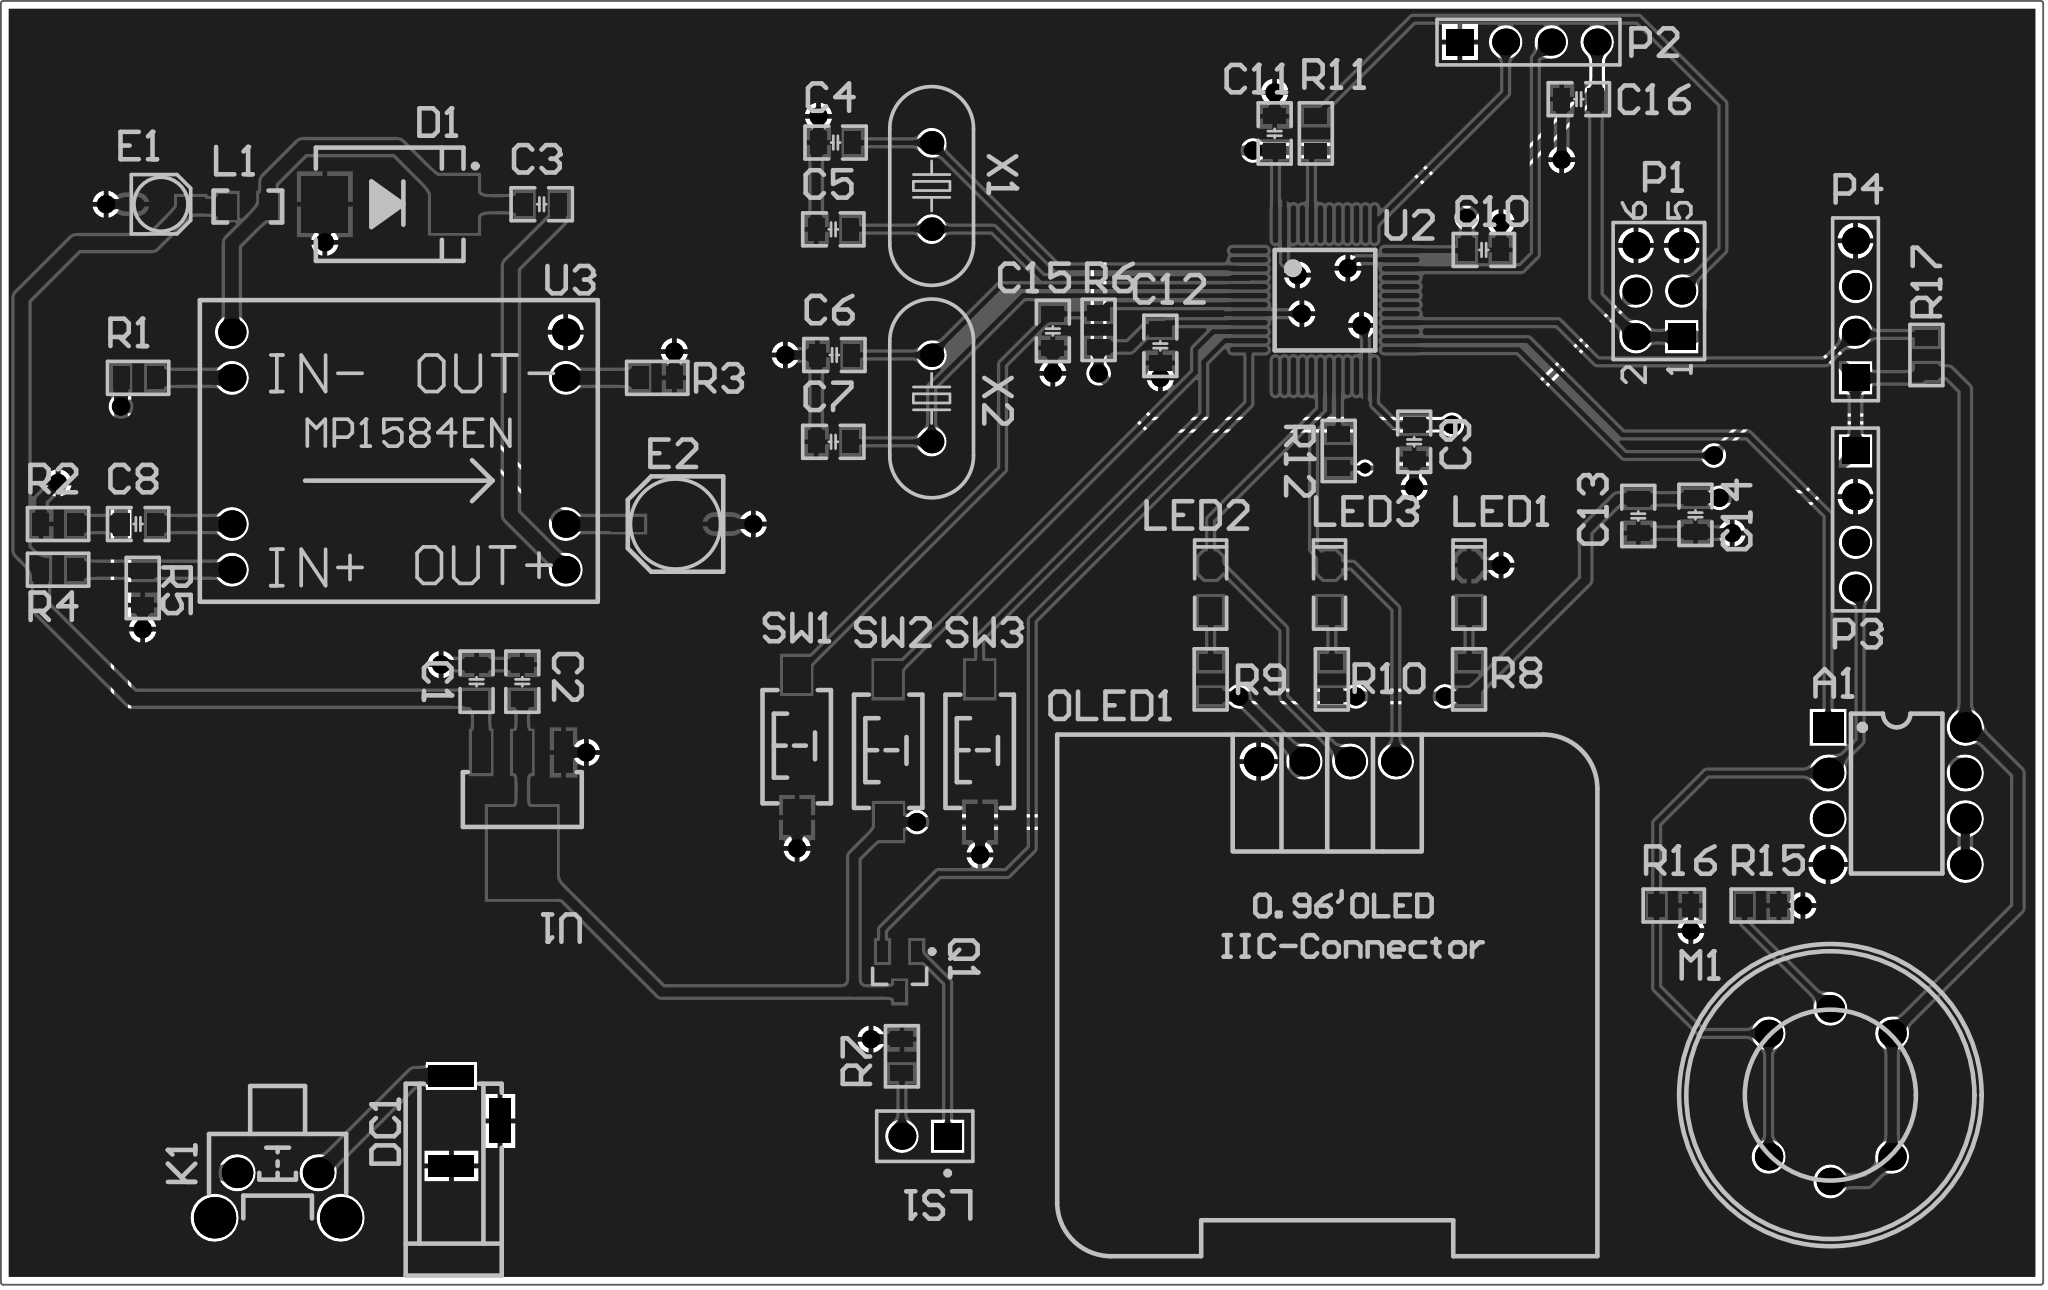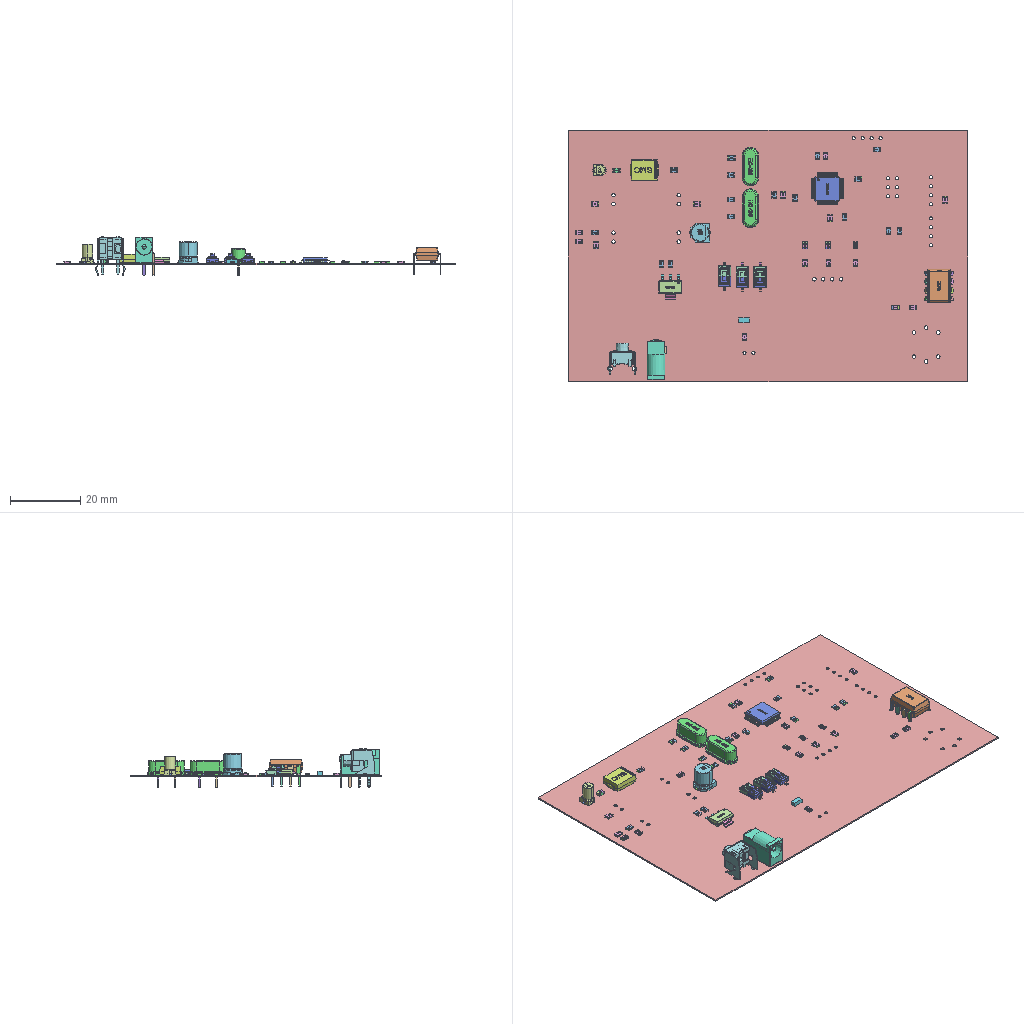Circuit board layout | Altium Designer | box 113.4 x 71.4 x 10.9 mm
Layer stack:
# Altium Designer layer stack of  (unit mm; dielectric type: 0 none, 1 core, 2 prepreg, 3 surface material)
index,name,kind,layer,copper_thickness_mm,dielectric_type,dielectric_thickness_mm,dielectric_material,dielectric_constant
0,Top Paste,other,,,,,,
1,Top Overlay,other,,,,,,
2,Top Solder,dielectric,,,3,0.0102,Solder Resist,3.5
3,Top Layer,copper,Top Layer,0.0356,,,,
4,Dielectric 1,dielectric,,,0,0.32,FR-4,4.8
5,Bottom Layer,copper,Bottom Layer,0.0356,,,,
6,Bottom Solder,dielectric,,,3,0.0102,Solder Resist,3.5
7,Bottom Overlay,other,,,,,,
8,Bottom Paste,other,,,,,,
# drill layer pairs: low layer,high layer
drill_pair,Top Layer,Bottom Layer
Part placement:
Designator,Comment,Layer,Footprint,Center-X(mm),Center-Y(mm),Rotation
R17,4.7K,TopLayer,R_0805_L,147.447,87.122,90
R16,1K,TopLayer,R_0805_L,133.416,56.515,0
R15,4.7K,TopLayer,R_0805_L,138.303,56.515,0
M1,MQ-2,TopLayer,MQ-2,142.113,45.974,0
A1,ADC0832,TopLayer,DIP8,145.796,62.611,360
C1,100nF,TopLayer,C_0805_L,66.929,68.961,270
C2,100nF,TopLayer,C_0805_L,69.469,68.961,270
C3,100nF,TopLayer,C_0805_L,70.546,95.504,0
C4,10PF,TopLayer,C_0805_L,86.868,98.933,0
C5,10PF,TopLayer,C_0805_L,86.741,94.107,0
C6,22PF,TopLayer,C_0805_L,86.802,87.122,0
C7,22PF,TopLayer,C_0805_L,86.741,82.296,0
C8,150PF,TopLayer,C_0805_L,48.133,77.724,0
C9,22UF,TopLayer,C_0805_L,118.999,82.296,90
C10,100nF,TopLayer,C_0805_L,122.87,92.964,180
C11,100nF,TopLayer,C_0805_L,111.252,99.441,270
C12,100nF,TopLayer,C_0805_L,104.902,87.63,90
C13,100nF,TopLayer,C_0805_L,131.445,78.171,90
C14,100nF,TopLayer,C_0805_L,134.62,78.232,90
C15,100nF,TopLayer,C_0805_L,98.933,88.458,90
C16,100nF,TopLayer,C_0805_L,128.143,101.346,0
D1,SS34,TopLayer,SMC,62.103,95.504,360
DC1,DC_Socket,TopLayer,DC-002,66.882,44.537,270
E1,22uF,TopLayer,CM_A(3*5.4),49.404,95.504,0
E2,220UF,TopLayer,CT_5*6_-_C,77.978,77.724,180
L1,15uH,TopLayer,L_0805,54.229,95.377,0
LED1,Red,TopLayer,LED_0805G,122.047,74.168,90
LED2,Red,TopLayer,LED_0805G,107.696,74.168,90
LED3,Red,TopLayer,LED_0805G,114.3,74.168,90
LS1,Speaker,TopLayer,PIN2,91.821,43.688,180
OLED1,0.96OLED_4P_MODULE_JX,TopLayer,0.96OLED_4P,114.173,64.517,0
P1,Header 3X2,TopLayer,HDR2X3,132.588,90.678,90
P2,Header 4,TopLayer,HDR1X4,125.349,104.521,360
P3,Header 4,TopLayer,HDR1X4,143.51,77.978,270
P4,Header 4,TopLayer,HDR1X4,143.51,89.662,90
Q1,PNP,TopLayer,SOT-23B_N,90.424,52.832,270
R1,100K,TopLayer,R_0805_L,48.133,85.852,0
R2,100K,TopLayer,R_0805_L,43.688,77.724,0
R3,100K,TopLayer,R_0805_L,76.962,85.852,180
R4,43K,TopLayer,R_0805_L,43.688,75.184,180
R5,8.2K,TopLayer,R_0805_L,48.387,74.168,90
R6,10K,TopLayer,R_0805_L,101.473,88.519,90
R7,20K,TopLayer,R_0805_L,90.551,48.133,90
R8,300,TopLayer,R_0805_L,122.047,69.088,270
R9,300,TopLayer,R_0805_L,107.696,69.088,270
R10,300,TopLayer,R_0805_L,114.427,69.088,270
R11,10K,TopLayer,R_0805_L,113.538,99.441,270
R12,10K,TopLayer,R_0805_L,114.808,81.788,270
SW1,3x6x5,TopLayer,TSW_SMD-3*6*2.5,84.719,65.376,90
SW2,3x6x5,TopLayer,TSW_SMD-3*6*2.5,89.799,65.122,90
SW3,3x6x5,TopLayer,TSW_SMD-3*6*2.5,94.879,65.122,90
U1,AMS1117,TopLayer,SOT223,69.469,62.23,180
U3,MP1584EN,TopLayer,MP1548EN,62.61,81.788,360
X1,32.768KHZ,TopLayer,OSC_HC-49S,92.202,96.52,270
X2,8MHZ,TopLayer,OSC_HC-49S,92.202,84.709,270
U2,STM32F103C8T6,TopLayer,LQFP48_7X7,114.033,90.17,270
K1,6x6x5,TopLayer,TSW_DIP-6*6*6_V,55.88,40.406,180
Pad and via stacks:
# Altium Designer via and pad stacks of  (unit mm). Each distinct definition once, with the count of objects using it.
# via: kind,start_layer,end_layer,hole_mm,diameter_mm,mode(0 simple;1 top-mid-bottom;2 full stack),diameter_per_layer,count,example_net
# pad: kind,layer,hole_mm,hole_type(0 round;1 square;2 slot),plating,top_size,top_shape(1 round;2 rect;3 octagon;9 rounded rect),mid_size,bottom_size,mode,footprint,size_per_layer,count,example
pad,Top Layer,0,0,plated,1.27x0.889,2,1.27x0.889,1.27x0.889,0,R 0805_L,,30,R17.1
pad,Top Layer,0,0,plated,1.27x0.889,2,1.27x0.889,1.27x0.889,0,C 0805_L,,32,C16.2
pad,Top Layer,0,0,plated,2x1.5,2,2x1.5,2x1.5,0,TSW SMD-3*6*2.5,,6,SW3.2
pad,Top Layer,0,0,plated,1.524x1.27,3,1.524x1.27,1.524x1.27,0,LED 0805G,,3,LED3.2
pad,Top Layer,0,0,plated,1.524x1.27,2,1.524x1.27,1.524x1.27,0,LED 0805G,,3,LED3.1
pad,Top Layer,0,0,plated,0.6x1.15,2,0.6x1.15,0.6x1.15,0,SOT-23B_N,,3,Q1.3
pad,Top Layer,0,0,plated,1.8x0.8,2,1.8x0.8,1.8x0.8,0,CT 5*6 - C,,1,E2.1
pad,Top Layer,0,0,plated,1.8x0.8,1,1.8x0.8,1.8x0.8,0,CT 5*6 - C,,1,E2.2
pad,Top Layer,0,0,plated,1.016x1.397,2,1.016x1.397,1.016x1.397,0,L 0805,,2,L1.1
pad,Top Layer,0,0,plated,1.5x0.8,1,1.5x0.8,1.5x0.8,0,CM A(3*5.4),,1,E1.2
pad,Top Layer,0,0,plated,1.5x0.8,2,1.5x0.8,1.5x0.8,0,CM A(3*5.4),,1,E1.1
pad,Top Layer,0,0,plated,3.15x2.6,2,3.15x2.6,3.15x2.6,0,SMC,,2,D1.2
pad,Top Layer,0,0,plated,3.81x5.08,2,3.81x5.08,3.81x5.08,0,SOT223,,1,U1.2
pad,Top Layer,0,0,plated,1.016x2.286,2,1.016x2.286,1.016x2.286,0,SOT223,,3,U1.2
pad,Top Layer,0,0,plated,0.3x2.1,1,0.3x2.1,0.3x2.1,0,LQFP48 7X7,,48,U2.1
pad,Multi-Layer,0.8,0,plated,1.7x1.7,1,1.7x1.7,1.7x1.7,0,DIP8,,7,A1.8
pad,Multi-Layer,0.8,0,plated,1.7x1.7,2,1.7x1.7,1.7x1.7,0,DIP8,,1,A1.1
pad,Multi-Layer,1,0,plated,1.524x1.524,1,1.524x1.524,1.524x1.524,0,MQ-2,,6,M1.6
pad,Multi-Layer,0.9,0,plated,1.5x1.5,2,1.5x1.5,1.5x1.5,0,HDR1X4,,3,P3.1
pad,Multi-Layer,0.9,0,plated,1.5x1.5,1,1.5x1.5,1.5x1.5,0,HDR1X4,,9,P3.2
pad,Multi-Layer,0.9,0,plated,1.5x1.5,1,1.5x1.5,1.5x1.5,0,HDR2X3,,5,P1.6
pad,Multi-Layer,0.9,0,plated,1.5x1.5,2,1.5x1.5,1.5x1.5,0,HDR2X3,,1,P1.1
pad,Multi-Layer,1,2,plated,1.65x1.65,1,1.65x1.65,1.65x1.65,0,0.96OLED_4P,,4,OLED1.4
pad,Multi-Layer,0.9,0,plated,1.5x1.5,1,1.5x1.5,1.5x1.5,0,PIN2,,1,LS1.2
pad,Multi-Layer,0.9,0,plated,1.5x1.5,2,1.5x1.5,1.5x1.5,0,PIN2,,1,LS1.1
pad,Multi-Layer,1,0,plated,1.524x1.524,1,1.524x1.524,1.524x1.524,0,MP1548EN,,8,U3.8
pad,Multi-Layer,0.6,0,plated,1.3x1.3,1,1.3x1.3,1.3x1.3,0,OSC HC-49S,,4,X1.1
pad,Multi-Layer,0.6,2,plated,2.5x1.2,2,2.5x1.2,2.5x1.2,0,DC-002,,3,DC1.1
pad,Multi-Layer,1.3,0,plated,2.3x2.3,1,2.3x2.3,2.3x2.3,0,TSW DIP-6*6*6_V,,2,K1.0
pad,Multi-Layer,0.9,0,plated,1.7x1.7,1,1.7x1.7,1.7x1.7,0,TSW DIP-6*6*6_V,,2,K1.1
via,Top Layer,Bottom Layer,0.508,1.016,0,,38,GND
via,Top Layer,Bottom Layer,0.3048,0.6096,0,,1,NetP1_4
Copper pours:
name,layer,net,type(0 solid;1 hatched;2 none)
G,Bottom Layer,GND,0
G,Top Layer,GND,0
Design rules, without the lines most boards share:
# Altium Designer design rules of  (exported by Altium Designer, unit mm)
# columns: name | kind | enabled | priority | scope1 | scope2 | descriptor | typed fields (field=value)
Clearance | 0 | enabled | 1 | All | All | Clearance Constraint (Gap=7mil) (All),(All) | gap=0.1778
PlaneConnect | 6 | enabled | 1 | All | All | Power Plane Connect Rule(Relief Connect )(Expansion=20mil) (Conductor Width=10mil) (Air Gap=10mil) (Entries=4) (All) | relief_conductor_width=0.254 relief_entries=4 relief_expansion=0.508
PolygonConnect | 20 | enabled | 1 | All | All | Polygon Connect Rule(Relief Connect )(Conductor Width=10mil) (Relief Angle=90 Angle) (Entries=4) (Air Gap Width=10mil) (All),(All) | connect_style(0=relief,1=direct,2=none)=0 relief_conductor_width=0.254 relief_entries=4
Width | 2 | enabled | 1 | All | All | Width Constraint (Min=10mil) (Max=30mil) (Preferred=10mil) (All) |
RoutingVias | 11 | enabled | 1 | All | All | Routing Via (MinHoleWidth=28mil) (MaxHoleWidth=28mil) (PreferredHoleWidth=28mil) (MinWidth=50mil) (MaxWidth=50mil) (PreferedWidth=50mil) (All) | via_min_hole=0.7112 via_max_hole=0.7112 via_preferred_diameter=1.27 via_preferred_hole=0.7112
PasteMaskExpansion | 14 | enabled | 1 | All | All | Paste Mask Expansion (Expansion =0mil) (All) | expansion=0
SolderMaskExpansion | 13 | enabled | 1 | All | All | Solder Mask Expansion (Expansion =4mil) (All) | expansion=0.1016
HoleSize | 42 | enabled | 1 | All | All | Hole Size Constraint (Min=1mil) (Max=3333mil) (All) |
DiffPairsRouting | 51 | enabled | 1 | All | All | Differential Pairs Uncoupled Length using the Gap Constraints (Min=10mil) (Max=10mil) (Prefered=10mil)  and Width Constraints (Min=15mil) (Max=15mil) (Prefered=15mil) (All) |
HoleToHoleClearance | 52 | enabled | 1 | All | All | Hole To Hole Clearance (Gap=10mil) (All),(All) | gap=0.254
MinimumSolderMaskSliver | 53 | enabled | 1 | All | All | Minimum Solder Mask Sliver (Gap=0mil) (All),(All) |
SilkToSolderMaskClearance | 54 | enabled | 1 | IsPad | All | Silk To Solder Mask (Clearance=0mil) (IsPad),(All) |
SilkToSilkClearance | 55 | enabled | 1 | All | All | Silk to Silk (Clearance=0mil) (All),(All) |
Classes set for this board:
# Altium Designer classes of  (member kind: 0 net, 1 component, 2 from-to, 3 pad, 4 layer, 5 differential pair, 6 design channel, 7 polygon, 8 structure, 9 xSignal)
# columns: class name | member kind | superclass | members
Sheet1 | 1 | no | C1; C2; C3; C4; C5; C6; C7; C8; C9; C10; C11; C12; C13; C14; C15; C16; D1; DC1; E1; E2; L1; LED1; LED2; LED3; LS1; OLED1; P1; P2; P3; P4; Q1; R1; R2; R3; R4; R5; R6; R7; R8; R9; R10; R11; R12; SW1; SW2; SW3; U1; U2; U3; X1; X2; U2; K1; A1; R15; R16; R17; M1;